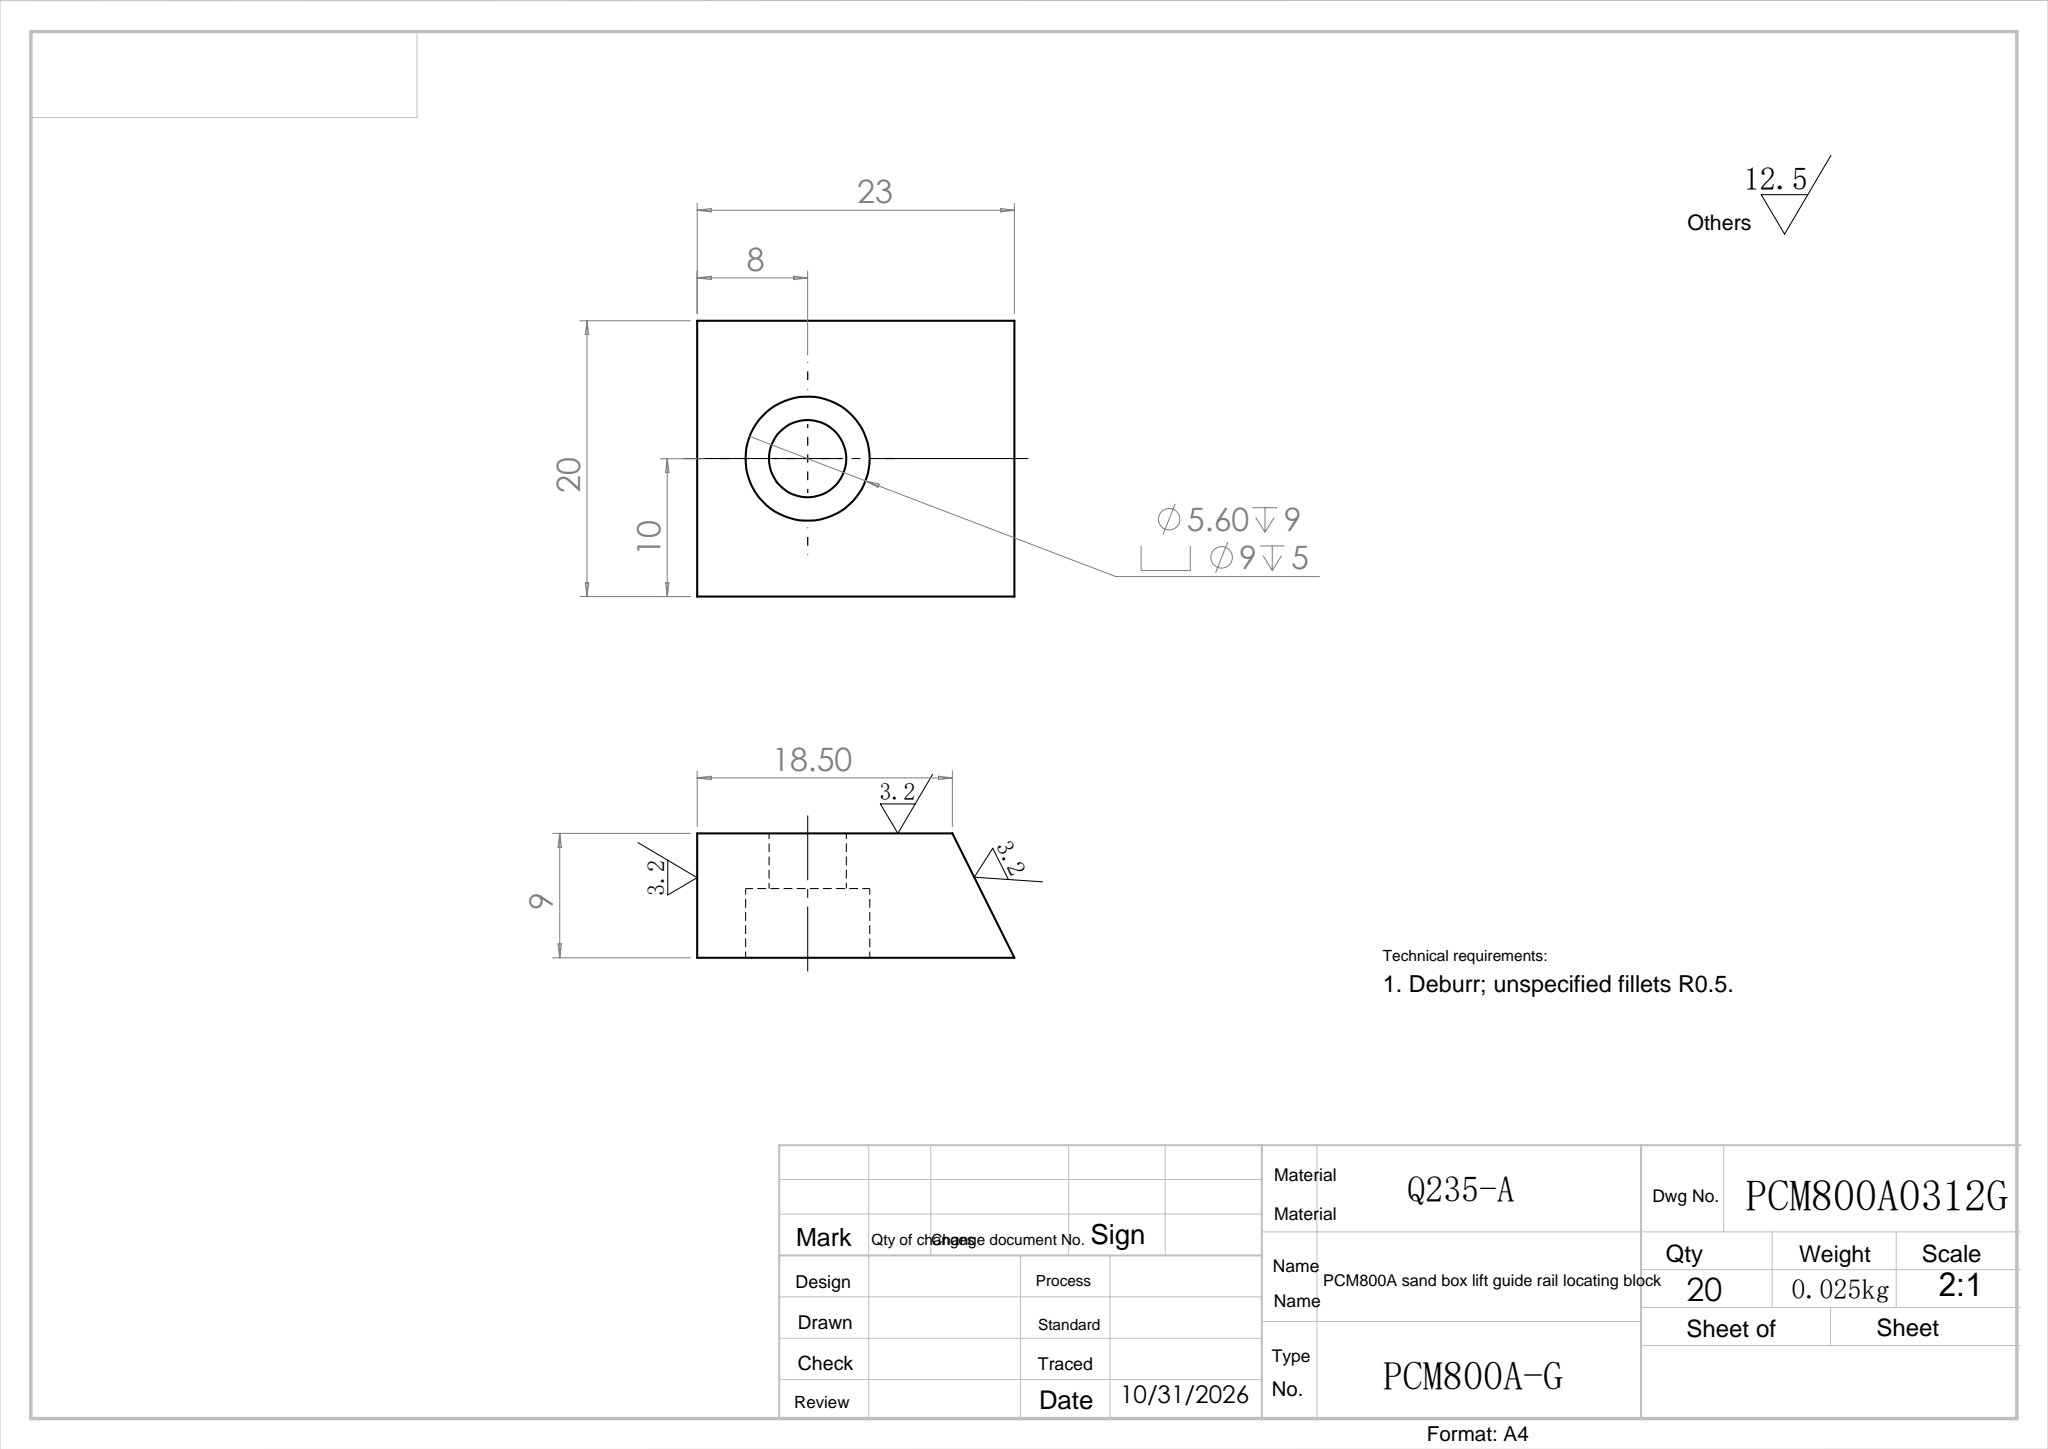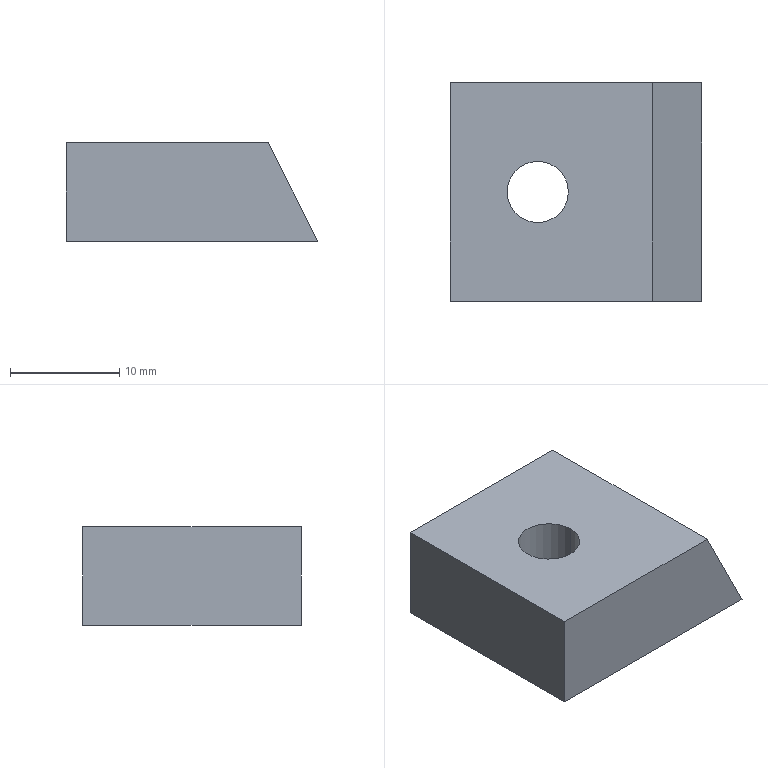Part | SolidWorks | features Cut 2, Extrusion 1 | 1 solid | 11 faces | box 23 x 20 x 9 mm | volume 3318 mm3 | plane 7 | cylinder 4 | commonest cylinder face diameters 5.6 x2 9 x2
STEP:
#1=CARTESIAN_POINT('',(10.8,10.,0.));
#2=VERTEX_POINT('',#1);
#3=CARTESIAN_POINT('',(5.2,10.,0.));
#4=VERTEX_POINT('',#3);
#5=CARTESIAN_POINT('',(8.,10.,0.));
#6=DIRECTION('',(0.,0.,-1.));
#7=DIRECTION('',(-1.,0.,0.));
#8=AXIS2_PLACEMENT_3D('',#5,#6,#7);
#9=CIRCLE('',#8,2.8);
#10=EDGE_CURVE('',#2,#4,#9,.T.);
#11=ORIENTED_EDGE('',*,*,#10,.F.);
#12=CARTESIAN_POINT('',(10.8,10.,-4.));
#13=VERTEX_POINT('',#12);
#14=CARTESIAN_POINT('',(10.8,10.,0.));
#15=DIRECTION('',(0.,0.,-1.));
#16=VECTOR('',#15,1000.);
#17=LINE('',#14,#16);
#18=EDGE_CURVE('',#2,#13,#17,.T.);
#19=ORIENTED_EDGE('',*,*,#18,.T.);
#20=CARTESIAN_POINT('',(5.2,10.,-4.));
#21=VERTEX_POINT('',#20);
#22=CARTESIAN_POINT('',(8.,10.,-4.));
#23=DIRECTION('',(0.,0.,-1.));
#24=DIRECTION('',(-1.,0.,0.));
#25=AXIS2_PLACEMENT_3D('',#22,#23,#24);
#26=CIRCLE('',#25,2.8);
#27=EDGE_CURVE('',#13,#21,#26,.T.);
#28=ORIENTED_EDGE('',*,*,#27,.T.);
#29=CARTESIAN_POINT('',(5.2,10.,0.));
#30=DIRECTION('',(0.,0.,-1.));
#31=VECTOR('',#30,1000.);
#32=LINE('',#29,#31);
#33=EDGE_CURVE('',#4,#21,#32,.T.);
#34=ORIENTED_EDGE('',*,*,#33,.F.);
#35=EDGE_LOOP('',(#11,#19,#28,#34));
#36=FACE_OUTER_BOUND('',#35,.T.);
#37=CARTESIAN_POINT('',(8.,10.,0.));
#38=DIRECTION('',(0.,0.,-1.));
#39=DIRECTION('',(-1.,0.,0.));
#40=AXIS2_PLACEMENT_3D('',#37,#38,#39);
#41=CYLINDRICAL_SURFACE('',#40,2.8);
#42=ADVANCED_FACE('',(#36),#41,.F.);
#43=CARTESIAN_POINT('',(12.5,10.,-4.));
#44=VERTEX_POINT('',#43);
#45=CARTESIAN_POINT('',(3.5,10.,-4.));
#46=VERTEX_POINT('',#45);
#47=CARTESIAN_POINT('',(8.,10.,-4.));
#48=DIRECTION('',(0.,0.,-1.));
#49=DIRECTION('',(-1.,0.,0.));
#50=AXIS2_PLACEMENT_3D('',#47,#48,#49);
#51=CIRCLE('',#50,4.5);
#52=EDGE_CURVE('',#44,#46,#51,.T.);
#53=ORIENTED_EDGE('',*,*,#52,.F.);
#54=CARTESIAN_POINT('',(12.5,10.,-9.));
#55=VERTEX_POINT('',#54);
#56=CARTESIAN_POINT('',(12.5,10.,-4.));
#57=DIRECTION('',(0.,0.,-1.));
#58=VECTOR('',#57,1000.);
#59=LINE('',#56,#58);
#60=EDGE_CURVE('',#44,#55,#59,.T.);
#61=ORIENTED_EDGE('',*,*,#60,.T.);
#62=CARTESIAN_POINT('',(3.5,10.,-9.));
#63=VERTEX_POINT('',#62);
#64=CARTESIAN_POINT('',(8.,10.,-9.));
#65=DIRECTION('',(0.,0.,-1.));
#66=DIRECTION('',(-1.,0.,0.));
#67=AXIS2_PLACEMENT_3D('',#64,#65,#66);
#68=CIRCLE('',#67,4.5);
#69=EDGE_CURVE('',#55,#63,#68,.T.);
#70=ORIENTED_EDGE('',*,*,#69,.T.);
#71=CARTESIAN_POINT('',(3.5,10.,-4.));
#72=DIRECTION('',(0.,0.,-1.));
#73=VECTOR('',#72,1000.);
#74=LINE('',#71,#73);
#75=EDGE_CURVE('',#46,#63,#74,.T.);
#76=ORIENTED_EDGE('',*,*,#75,.F.);
#77=EDGE_LOOP('',(#53,#61,#70,#76));
#78=FACE_OUTER_BOUND('',#77,.T.);
#79=CARTESIAN_POINT('',(8.,10.,-4.));
#80=DIRECTION('',(0.,0.,-1.));
#81=DIRECTION('',(-1.,0.,0.));
#82=AXIS2_PLACEMENT_3D('',#79,#80,#81);
#83=CYLINDRICAL_SURFACE('',#82,4.5);
#84=ADVANCED_FACE('',(#78),#83,.F.);
#85=CARTESIAN_POINT('',(0.,0.,-9.));
#86=VERTEX_POINT('',#85);
#87=CARTESIAN_POINT('',(0.,0.,0.));
#88=VERTEX_POINT('',#87);
#89=CARTESIAN_POINT('',(0.,0.,0.));
#90=DIRECTION('',(0.,0.,1.));
#91=VECTOR('',#90,1000.);
#92=LINE('',#89,#91);
#93=EDGE_CURVE('',#86,#88,#92,.T.);
#94=ORIENTED_EDGE('',*,*,#93,.T.);
#95=CARTESIAN_POINT('',(0.,20.,0.));
#96=VERTEX_POINT('',#95);
#97=CARTESIAN_POINT('',(0.,20.,0.));
#98=DIRECTION('',(0.,-1.,0.));
#99=VECTOR('',#98,1000.);
#100=LINE('',#97,#99);
#101=EDGE_CURVE('',#96,#88,#100,.T.);
#102=ORIENTED_EDGE('',*,*,#101,.F.);
#103=CARTESIAN_POINT('',(0.,20.,-9.));
#104=VERTEX_POINT('',#103);
#105=CARTESIAN_POINT('',(0.,20.,0.));
#106=DIRECTION('',(0.,0.,1.));
#107=VECTOR('',#106,1000.);
#108=LINE('',#105,#107);
#109=EDGE_CURVE('',#104,#96,#108,.T.);
#110=ORIENTED_EDGE('',*,*,#109,.F.);
#111=CARTESIAN_POINT('',(0.,20.,-9.));
#112=DIRECTION('',(0.,-1.,0.));
#113=VECTOR('',#112,1000.);
#114=LINE('',#111,#113);
#115=EDGE_CURVE('',#104,#86,#114,.T.);
#116=ORIENTED_EDGE('',*,*,#115,.T.);
#117=EDGE_LOOP('',(#94,#102,#110,#116));
#118=FACE_OUTER_BOUND('',#117,.T.);
#119=CARTESIAN_POINT('',(0.,20.,0.));
#120=DIRECTION('',(1.,0.,0.));
#121=DIRECTION('',(0.,0.,-1.));
#122=AXIS2_PLACEMENT_3D('',#119,#120,#121);
#123=PLANE('',#122);
#124=ADVANCED_FACE('',(#118),#123,.F.);
#125=CARTESIAN_POINT('',(8.,10.,0.));
#126=DIRECTION('',(0.,0.,-1.));
#127=DIRECTION('',(-1.,0.,0.));
#128=AXIS2_PLACEMENT_3D('',#125,#126,#127);
#129=CIRCLE('',#128,2.8);
#130=EDGE_CURVE('',#4,#2,#129,.T.);
#131=ORIENTED_EDGE('',*,*,#130,.T.);
#132=ORIENTED_EDGE('',*,*,#10,.T.);
#133=EDGE_LOOP('',(#131,#132));
#134=FACE_BOUND('',#133,.T.);
#135=CARTESIAN_POINT('',(18.5,0.,0.));
#136=VERTEX_POINT('',#135);
#137=CARTESIAN_POINT('',(0.,0.,0.));
#138=DIRECTION('',(1.,0.,0.));
#139=VECTOR('',#138,1000.);
#140=LINE('',#137,#139);
#141=EDGE_CURVE('',#88,#136,#140,.T.);
#142=ORIENTED_EDGE('',*,*,#141,.T.);
#143=CARTESIAN_POINT('',(18.5,20.,0.));
#144=VERTEX_POINT('',#143);
#145=CARTESIAN_POINT('',(18.5,20.,0.));
#146=DIRECTION('',(0.,-1.,0.));
#147=VECTOR('',#146,1000.);
#148=LINE('',#145,#147);
#149=EDGE_CURVE('',#144,#136,#148,.T.);
#150=ORIENTED_EDGE('',*,*,#149,.F.);
#151=CARTESIAN_POINT('',(0.,20.,0.));
#152=DIRECTION('',(1.,0.,0.));
#153=VECTOR('',#152,1000.);
#154=LINE('',#151,#153);
#155=EDGE_CURVE('',#96,#144,#154,.T.);
#156=ORIENTED_EDGE('',*,*,#155,.F.);
#157=ORIENTED_EDGE('',*,*,#101,.T.);
#158=EDGE_LOOP('',(#142,#150,#156,#157));
#159=FACE_OUTER_BOUND('',#158,.T.);
#160=CARTESIAN_POINT('',(0.,20.,0.));
#161=DIRECTION('',(0.,0.,-1.));
#162=DIRECTION('',(-1.,0.,0.));
#163=AXIS2_PLACEMENT_3D('',#160,#161,#162);
#164=PLANE('',#163);
#165=ADVANCED_FACE('',(#134,#159),#164,.F.);
#166=CARTESIAN_POINT('',(23.,0.,-9.));
#167=VERTEX_POINT('',#166);
#168=CARTESIAN_POINT('',(18.5,0.,0.));
#169=DIRECTION('',(0.4472,0.,-0.8944));
#170=VECTOR('',#169,1000.);
#171=LINE('',#168,#170);
#172=EDGE_CURVE('',#136,#167,#171,.T.);
#173=ORIENTED_EDGE('',*,*,#172,.T.);
#174=CARTESIAN_POINT('',(23.,20.,-9.));
#175=VERTEX_POINT('',#174);
#176=CARTESIAN_POINT('',(23.,20.,-9.));
#177=DIRECTION('',(0.,-1.,0.));
#178=VECTOR('',#177,1000.);
#179=LINE('',#176,#178);
#180=EDGE_CURVE('',#175,#167,#179,.T.);
#181=ORIENTED_EDGE('',*,*,#180,.F.);
#182=CARTESIAN_POINT('',(18.5,20.,0.));
#183=DIRECTION('',(0.4472,0.,-0.8944));
#184=VECTOR('',#183,1000.);
#185=LINE('',#182,#184);
#186=EDGE_CURVE('',#144,#175,#185,.T.);
#187=ORIENTED_EDGE('',*,*,#186,.F.);
#188=ORIENTED_EDGE('',*,*,#149,.T.);
#189=EDGE_LOOP('',(#173,#181,#187,#188));
#190=FACE_OUTER_BOUND('',#189,.T.);
#191=CARTESIAN_POINT('',(18.5,20.,0.));
#192=DIRECTION('',(-0.8944,0.,-0.4472));
#193=DIRECTION('',(-0.4472,0.,0.8944));
#194=AXIS2_PLACEMENT_3D('',#191,#192,#193);
#195=PLANE('',#194);
#196=ADVANCED_FACE('',(#190),#195,.F.);
#197=CARTESIAN_POINT('',(8.,10.,-9.));
#198=DIRECTION('',(0.,0.,-1.));
#199=DIRECTION('',(-1.,0.,0.));
#200=AXIS2_PLACEMENT_3D('',#197,#198,#199);
#201=CIRCLE('',#200,4.5);
#202=EDGE_CURVE('',#63,#55,#201,.T.);
#203=ORIENTED_EDGE('',*,*,#202,.F.);
#204=ORIENTED_EDGE('',*,*,#69,.F.);
#205=EDGE_LOOP('',(#203,#204));
#206=FACE_BOUND('',#205,.T.);
#207=CARTESIAN_POINT('',(0.,0.,-9.));
#208=DIRECTION('',(-1.,0.,0.));
#209=VECTOR('',#208,1000.);
#210=LINE('',#207,#209);
#211=EDGE_CURVE('',#167,#86,#210,.T.);
#212=ORIENTED_EDGE('',*,*,#211,.T.);
#213=ORIENTED_EDGE('',*,*,#115,.F.);
#214=CARTESIAN_POINT('',(0.,20.,-9.));
#215=DIRECTION('',(-1.,0.,0.));
#216=VECTOR('',#215,1000.);
#217=LINE('',#214,#216);
#218=EDGE_CURVE('',#175,#104,#217,.T.);
#219=ORIENTED_EDGE('',*,*,#218,.F.);
#220=ORIENTED_EDGE('',*,*,#180,.T.);
#221=EDGE_LOOP('',(#212,#213,#219,#220));
#222=FACE_OUTER_BOUND('',#221,.T.);
#223=CARTESIAN_POINT('',(0.,20.,-9.));
#224=DIRECTION('',(0.,0.,1.));
#225=DIRECTION('',(1.,0.,0.));
#226=AXIS2_PLACEMENT_3D('',#223,#224,#225);
#227=PLANE('',#226);
#228=ADVANCED_FACE('',(#206,#222),#227,.F.);
#229=ORIENTED_EDGE('',*,*,#109,.T.);
#230=ORIENTED_EDGE('',*,*,#155,.T.);
#231=ORIENTED_EDGE('',*,*,#186,.T.);
#232=ORIENTED_EDGE('',*,*,#218,.T.);
#233=EDGE_LOOP('',(#229,#230,#231,#232));
#234=FACE_OUTER_BOUND('',#233,.T.);
#235=CARTESIAN_POINT('',(0.,20.,-9.));
#236=DIRECTION('',(0.,-1.,0.));
#237=DIRECTION('',(0.,0.,-1.));
#238=AXIS2_PLACEMENT_3D('',#235,#236,#237);
#239=PLANE('',#238);
#240=ADVANCED_FACE('',(#234),#239,.F.);
#241=ORIENTED_EDGE('',*,*,#93,.F.);
#242=ORIENTED_EDGE('',*,*,#211,.F.);
#243=ORIENTED_EDGE('',*,*,#172,.F.);
#244=ORIENTED_EDGE('',*,*,#141,.F.);
#245=EDGE_LOOP('',(#241,#242,#243,#244));
#246=FACE_OUTER_BOUND('',#245,.T.);
#247=CARTESIAN_POINT('',(0.,0.,-9.));
#248=DIRECTION('',(0.,-1.,0.));
#249=DIRECTION('',(0.,0.,-1.));
#250=AXIS2_PLACEMENT_3D('',#247,#248,#249);
#251=PLANE('',#250);
#252=ADVANCED_FACE('',(#246),#251,.T.);
#253=ORIENTED_EDGE('',*,*,#60,.F.);
#254=CARTESIAN_POINT('',(8.,10.,-4.));
#255=DIRECTION('',(0.,0.,-1.));
#256=DIRECTION('',(-1.,0.,0.));
#257=AXIS2_PLACEMENT_3D('',#254,#255,#256);
#258=CIRCLE('',#257,4.5);
#259=EDGE_CURVE('',#46,#44,#258,.T.);
#260=ORIENTED_EDGE('',*,*,#259,.F.);
#261=ORIENTED_EDGE('',*,*,#75,.T.);
#262=ORIENTED_EDGE('',*,*,#202,.T.);
#263=EDGE_LOOP('',(#253,#260,#261,#262));
#264=FACE_OUTER_BOUND('',#263,.T.);
#265=CARTESIAN_POINT('',(8.,10.,-4.));
#266=DIRECTION('',(0.,0.,-1.));
#267=DIRECTION('',(-1.,0.,0.));
#268=AXIS2_PLACEMENT_3D('',#265,#266,#267);
#269=CYLINDRICAL_SURFACE('',#268,4.5);
#270=ADVANCED_FACE('',(#264),#269,.F.);
#271=CARTESIAN_POINT('',(8.,10.,-4.));
#272=DIRECTION('',(0.,0.,-1.));
#273=DIRECTION('',(-1.,0.,0.));
#274=AXIS2_PLACEMENT_3D('',#271,#272,#273);
#275=CIRCLE('',#274,2.8);
#276=EDGE_CURVE('',#21,#13,#275,.T.);
#277=ORIENTED_EDGE('',*,*,#276,.F.);
#278=ORIENTED_EDGE('',*,*,#27,.F.);
#279=EDGE_LOOP('',(#277,#278));
#280=FACE_BOUND('',#279,.T.);
#281=ORIENTED_EDGE('',*,*,#259,.T.);
#282=ORIENTED_EDGE('',*,*,#52,.T.);
#283=EDGE_LOOP('',(#281,#282));
#284=FACE_OUTER_BOUND('',#283,.T.);
#285=CARTESIAN_POINT('',(8.,10.,-4.));
#286=DIRECTION('',(0.,0.,-1.));
#287=DIRECTION('',(-1.,0.,0.));
#288=AXIS2_PLACEMENT_3D('',#285,#286,#287);
#289=PLANE('',#288);
#290=ADVANCED_FACE('',(#280,#284),#289,.T.);
#291=ORIENTED_EDGE('',*,*,#18,.F.);
#292=ORIENTED_EDGE('',*,*,#130,.F.);
#293=ORIENTED_EDGE('',*,*,#33,.T.);
#294=ORIENTED_EDGE('',*,*,#276,.T.);
#295=EDGE_LOOP('',(#291,#292,#293,#294));
#296=FACE_OUTER_BOUND('',#295,.T.);
#297=CARTESIAN_POINT('',(8.,10.,0.));
#298=DIRECTION('',(0.,0.,-1.));
#299=DIRECTION('',(-1.,0.,0.));
#300=AXIS2_PLACEMENT_3D('',#297,#298,#299);
#301=CYLINDRICAL_SURFACE('',#300,2.8);
#302=ADVANCED_FACE('',(#296),#301,.F.);
#303=CLOSED_SHELL('',(#42,#84,#124,#165,#196,#228,#240,#252,#270,#290,#302));
#304=MANIFOLD_SOLID_BREP('',#303);
#305=CARTESIAN_POINT('',(0.,0.,0.));
#306=DIRECTION('',(0.,0.,1.));
#307=DIRECTION('',(1.,0.,0.));
#308=AXIS2_PLACEMENT_3D('',#305,#306,#307);
#309=(LENGTH_UNIT()NAMED_UNIT(*)SI_UNIT(.MILLI.,.METRE.));
#310=UNCERTAINTY_MEASURE_WITH_UNIT(LENGTH_MEASURE(0.00001),#309,'','');
#311=(NAMED_UNIT(*)PLANE_ANGLE_UNIT()SI_UNIT($,.RADIAN.));
#312=(NAMED_UNIT(*)SI_UNIT($,.STERADIAN.)SOLID_ANGLE_UNIT());
#313=(GEOMETRIC_REPRESENTATION_CONTEXT(3)GLOBAL_UNCERTAINTY_ASSIGNED_CONTEXT((#310))GLOBAL_UNIT_ASSIGNED_CONTEXT((#309,#311,#312))REPRESENTATION_CONTEXT('',''));
#314=ADVANCED_BREP_SHAPE_REPRESENTATION('',(#304,#308),#313);